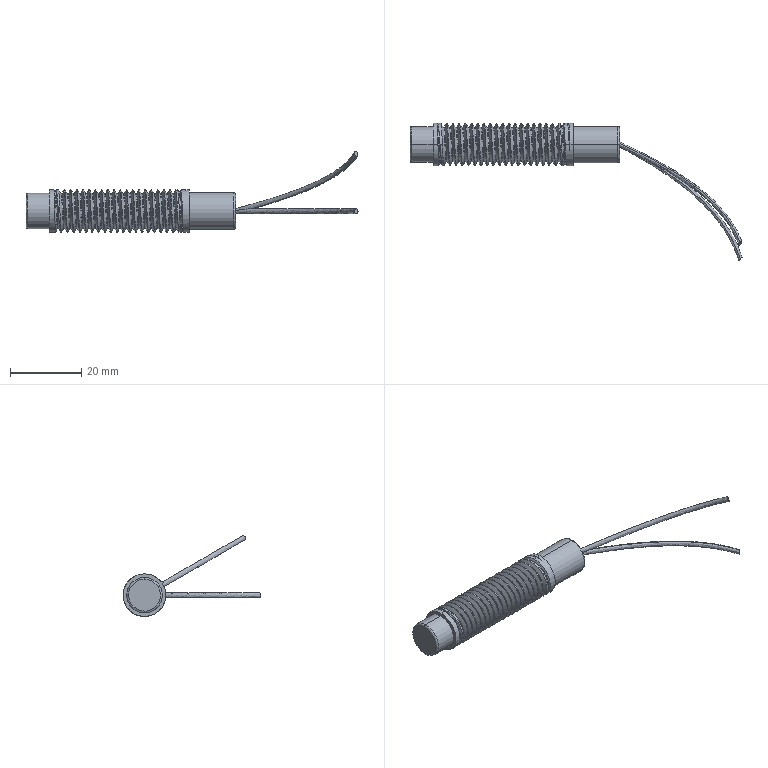Part | STEP file | 11-ganyingkaiguan11 | 1 solid | 83 faces | box 93.466 x 38.745 x 22.78 mm | volume 5435 mm3 | cylinder 48 | spline 29 | plane 6 | commonest cylinder face diameters 12 x44 10 x2 10.25 x2